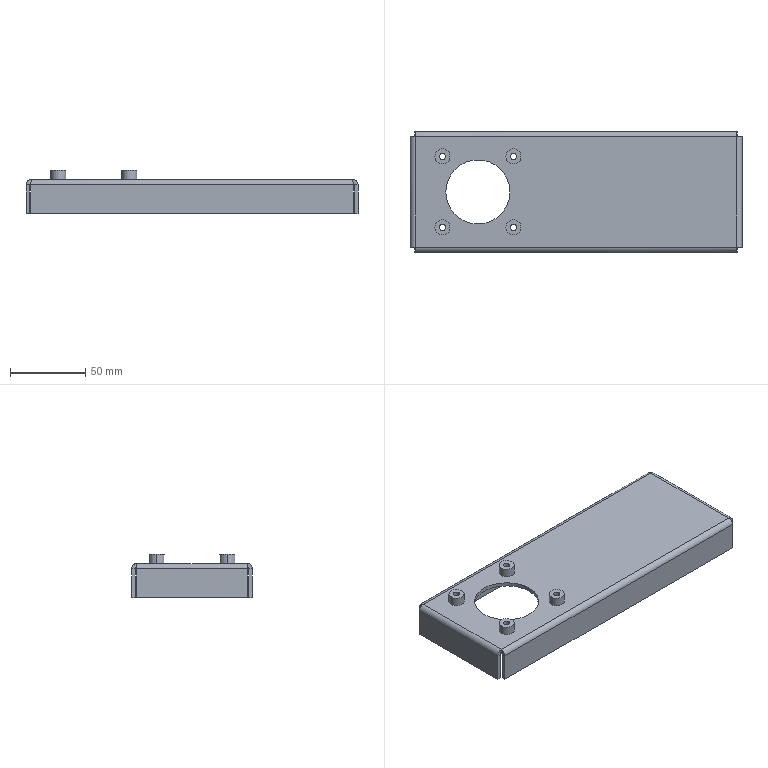Part | SolidWorks | features BaseBody 5 | 5 solids | 72 faces | box 220 x 80 x 28.5 mm | volume 68987 mm3 | cylinder 34 | plane 30 | spline 8 | commonest cylinder face diameters 4.2 x8 5.5 x8 10 x8 2 x4 7 x4 42.5 x2